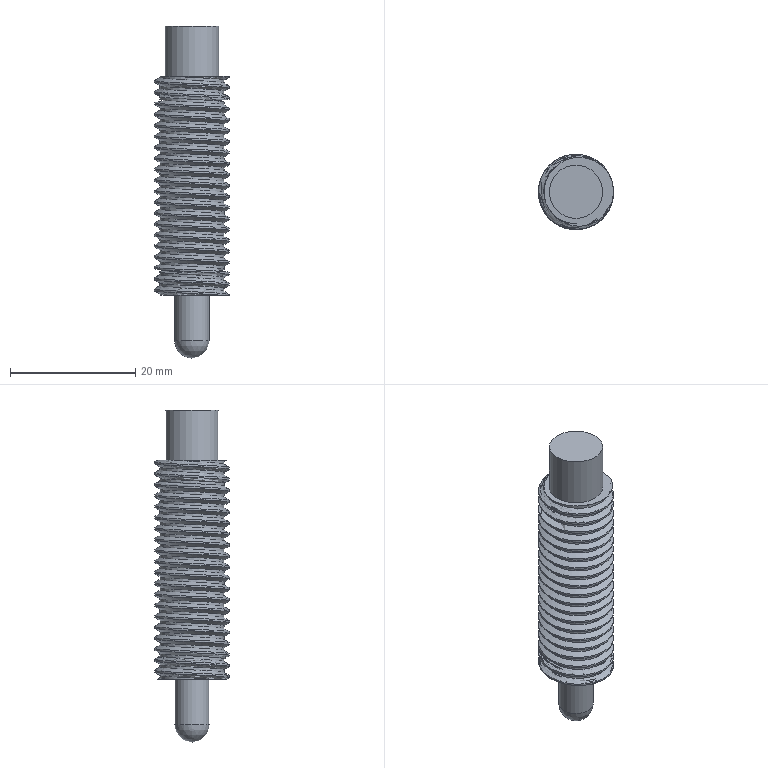Part | NX | features solid 2 | 1 solid | 10 faces | box 11.998 x 11.997 x 53 mm | volume 4026 mm3 | cylinder 4 | plane 3 | spline 2 | sphere 1 | commonest cylinder face diameters 5.5 x1 8.5 x1 10.25 x1 12 x1